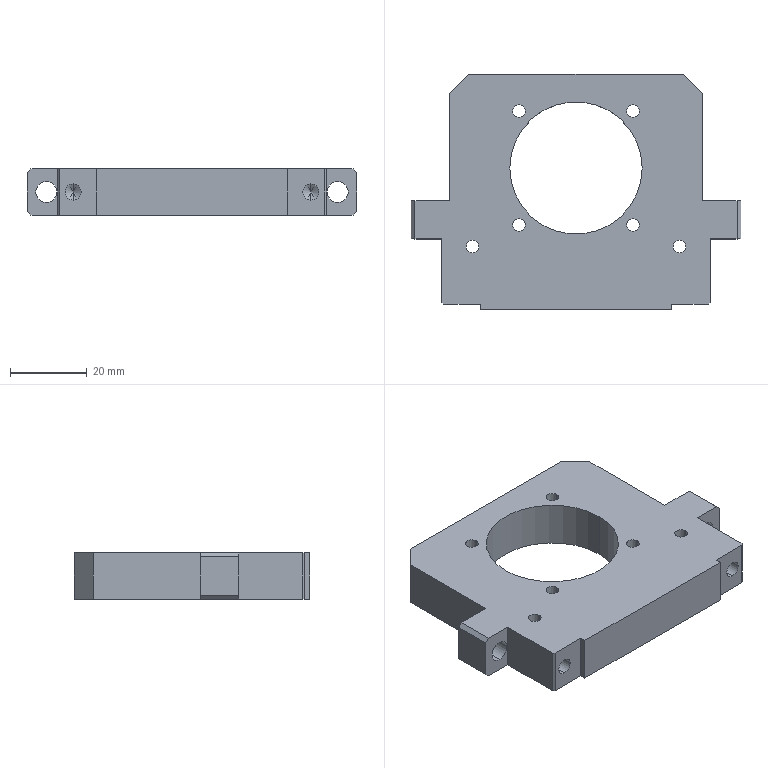Part | SolidWorks | features HoleWzd 5, ICE 5, Chamfer 4, MoveFace 3, Extrusion 1 | 1 solid | 66 faces | box 86 x 61.5 x 12 mm | volume 38021 mm3 | cylinder 30 | plane 28 | cone 8 | commonest cylinder face diameters 3.3 x16 4.2 x4 5.5 x4 9 x4 34.5 x2